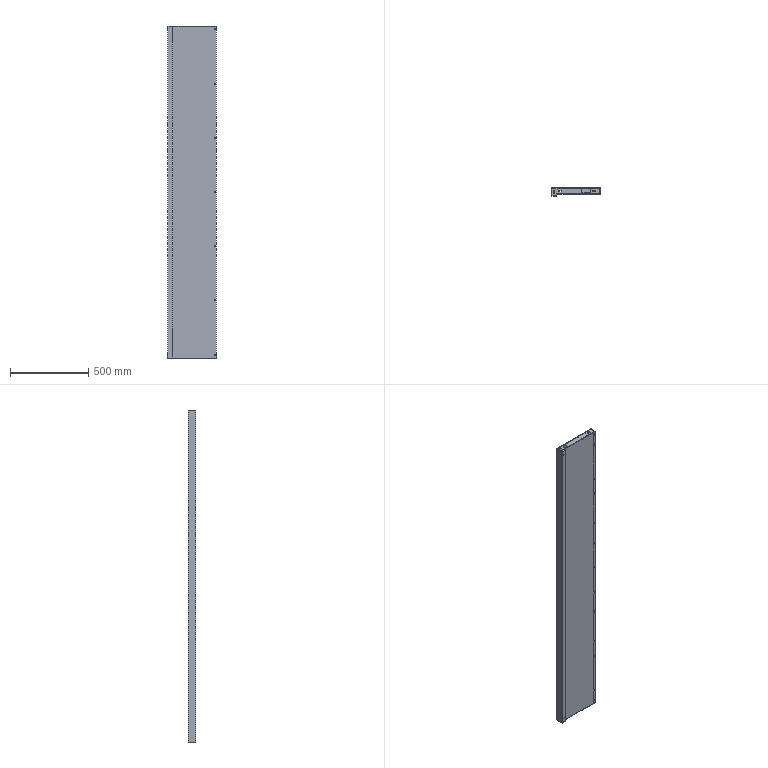Part | SolidWorks | 5 solids | 353 faces | box 310.7 x 50 x 2116 mm | volume 2074719 mm3 | plane 200 | cylinder 153 | commonest cylinder face diameters 5 x35 6.2 x28 10 x20 4.2 x14 8 x12 11 x12